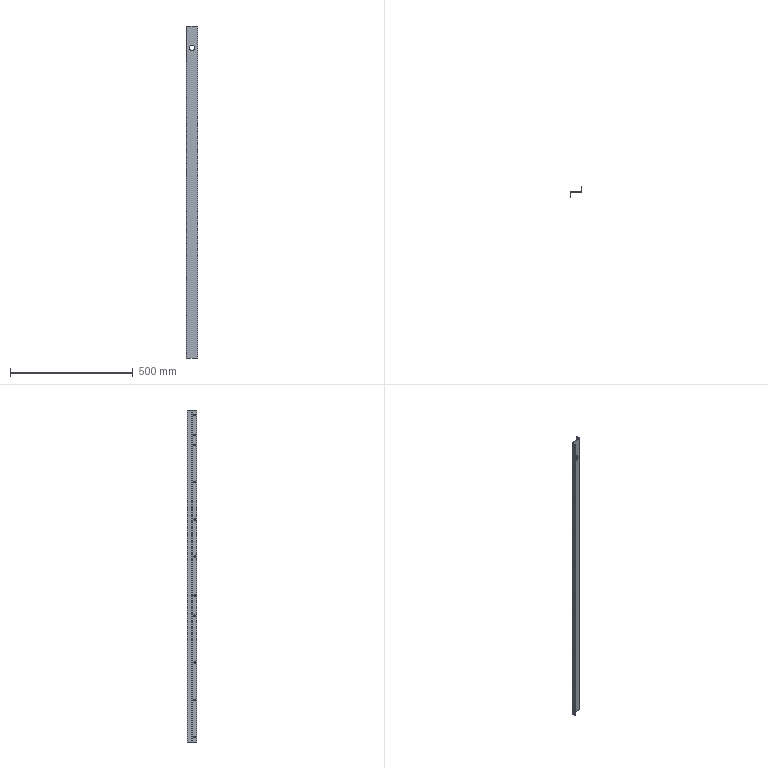Part | SolidWorks | features Cut 3, FlatPattern 1, SMBaseFlange 1, SheetMetal 1 | 1 solid | 46 faces | box 47.2 x 40 x 1350 mm | volume 135924 mm3 | cylinder 28 | plane 18 | commonest cylinder face diameters 6.5 x20 2.4 x2 4.8 x2 6.393 x2 22 x2
STEP:
#1=CARTESIAN_POINT('',(23.9,20.,1250.));
#2=VERTEX_POINT('',#1);
#3=CARTESIAN_POINT('',(23.9,20.,1272.));
#4=VERTEX_POINT('',#3);
#5=CARTESIAN_POINT('',(23.9,20.,1261.));
#6=DIRECTION('',(0.,1.,0.));
#7=DIRECTION('',(0.,0.,1.));
#8=AXIS2_PLACEMENT_3D('',#5,#6,#7);
#9=CIRCLE('',#8,11.);
#10=EDGE_CURVE('',#2,#4,#9,.T.);
#11=ORIENTED_EDGE('',*,*,#10,.T.);
#12=CARTESIAN_POINT('',(23.9,18.8,1272.));
#13=VERTEX_POINT('',#12);
#14=CARTESIAN_POINT('',(23.9,20.8,1272.));
#15=DIRECTION('',(0.,-1.,0.));
#16=VECTOR('',#15,1000.);
#17=LINE('',#14,#16);
#18=EDGE_CURVE('',#4,#13,#17,.T.);
#19=ORIENTED_EDGE('',*,*,#18,.T.);
#20=CARTESIAN_POINT('',(23.9,18.8,1250.));
#21=VERTEX_POINT('',#20);
#22=CARTESIAN_POINT('',(23.9,18.8,1261.));
#23=DIRECTION('',(0.,-1.,0.));
#24=DIRECTION('',(0.,0.,-1.));
#25=AXIS2_PLACEMENT_3D('',#22,#23,#24);
#26=CIRCLE('',#25,11.);
#27=EDGE_CURVE('',#13,#21,#26,.T.);
#28=ORIENTED_EDGE('',*,*,#27,.T.);
#29=CARTESIAN_POINT('',(23.9,20.8,1250.));
#30=DIRECTION('',(0.,-1.,0.));
#31=VECTOR('',#30,1000.);
#32=LINE('',#29,#31);
#33=EDGE_CURVE('',#2,#21,#32,.T.);
#34=ORIENTED_EDGE('',*,*,#33,.F.);
#35=EDGE_LOOP('',(#11,#19,#28,#34));
#36=FACE_OUTER_BOUND('',#35,.T.);
#37=CARTESIAN_POINT('',(23.9,20.8,1261.));
#38=DIRECTION('',(0.,-1.,0.));
#39=DIRECTION('',(0.,0.,-1.));
#40=AXIS2_PLACEMENT_3D('',#37,#38,#39);
#41=CYLINDRICAL_SURFACE('',#40,11.);
#42=ADVANCED_FACE('',(#36),#41,.F.);
#43=CARTESIAN_POINT('',(0.,9.,16.75));
#44=VERTEX_POINT('',#43);
#45=CARTESIAN_POINT('',(0.,9.,23.25));
#46=VERTEX_POINT('',#45);
#47=CARTESIAN_POINT('',(0.,9.,20.));
#48=DIRECTION('',(-1.,0.,0.));
#49=DIRECTION('',(0.,0.,1.));
#50=AXIS2_PLACEMENT_3D('',#47,#48,#49);
#51=CIRCLE('',#50,3.25);
#52=EDGE_CURVE('',#44,#46,#51,.T.);
#53=ORIENTED_EDGE('',*,*,#52,.T.);
#54=CARTESIAN_POINT('',(1.2,9.,23.25));
#55=VERTEX_POINT('',#54);
#56=CARTESIAN_POINT('',(-8.8,9.,23.25));
#57=DIRECTION('',(1.,0.,0.));
#58=VECTOR('',#57,1000.);
#59=LINE('',#56,#58);
#60=EDGE_CURVE('',#46,#55,#59,.T.);
#61=ORIENTED_EDGE('',*,*,#60,.T.);
#62=CARTESIAN_POINT('',(1.2,9.,16.75));
#63=VERTEX_POINT('',#62);
#64=CARTESIAN_POINT('',(1.2,9.,20.));
#65=DIRECTION('',(1.,0.,0.));
#66=DIRECTION('',(0.,0.,1.));
#67=AXIS2_PLACEMENT_3D('',#64,#65,#66);
#68=CIRCLE('',#67,3.25);
#69=EDGE_CURVE('',#55,#63,#68,.T.);
#70=ORIENTED_EDGE('',*,*,#69,.T.);
#71=CARTESIAN_POINT('',(-8.8,9.,16.75));
#72=DIRECTION('',(1.,0.,0.));
#73=VECTOR('',#72,1000.);
#74=LINE('',#71,#73);
#75=EDGE_CURVE('',#44,#63,#74,.T.);
#76=ORIENTED_EDGE('',*,*,#75,.F.);
#77=EDGE_LOOP('',(#53,#61,#70,#76));
#78=FACE_OUTER_BOUND('',#77,.T.);
#79=CARTESIAN_POINT('',(-8.8,9.,20.));
#80=DIRECTION('',(1.,0.,0.));
#81=DIRECTION('',(0.,0.,-1.));
#82=AXIS2_PLACEMENT_3D('',#79,#80,#81);
#83=CYLINDRICAL_SURFACE('',#82,3.25);
#84=ADVANCED_FACE('',(#78),#83,.F.);
#85=CARTESIAN_POINT('',(0.,9.,166.75));
#86=VERTEX_POINT('',#85);
#87=CARTESIAN_POINT('',(0.,9.,173.25));
#88=VERTEX_POINT('',#87);
#89=CARTESIAN_POINT('',(0.,9.,170.));
#90=DIRECTION('',(-1.,0.,0.));
#91=DIRECTION('',(0.,0.,1.));
#92=AXIS2_PLACEMENT_3D('',#89,#90,#91);
#93=CIRCLE('',#92,3.25);
#94=EDGE_CURVE('',#86,#88,#93,.T.);
#95=ORIENTED_EDGE('',*,*,#94,.T.);
#96=CARTESIAN_POINT('',(1.2,9.,173.25));
#97=VERTEX_POINT('',#96);
#98=CARTESIAN_POINT('',(-8.8,9.,173.25));
#99=DIRECTION('',(1.,0.,0.));
#100=VECTOR('',#99,1000.);
#101=LINE('',#98,#100);
#102=EDGE_CURVE('',#88,#97,#101,.T.);
#103=ORIENTED_EDGE('',*,*,#102,.T.);
#104=CARTESIAN_POINT('',(1.2,9.,166.75));
#105=VERTEX_POINT('',#104);
#106=CARTESIAN_POINT('',(1.2,9.,170.));
#107=DIRECTION('',(1.,0.,0.));
#108=DIRECTION('',(0.,0.,1.));
#109=AXIS2_PLACEMENT_3D('',#106,#107,#108);
#110=CIRCLE('',#109,3.25);
#111=EDGE_CURVE('',#97,#105,#110,.T.);
#112=ORIENTED_EDGE('',*,*,#111,.T.);
#113=CARTESIAN_POINT('',(-8.8,9.,166.75));
#114=DIRECTION('',(1.,0.,0.));
#115=VECTOR('',#114,1000.);
#116=LINE('',#113,#115);
#117=EDGE_CURVE('',#86,#105,#116,.T.);
#118=ORIENTED_EDGE('',*,*,#117,.F.);
#119=EDGE_LOOP('',(#95,#103,#112,#118));
#120=FACE_OUTER_BOUND('',#119,.T.);
#121=CARTESIAN_POINT('',(-8.8,9.,170.));
#122=DIRECTION('',(1.,0.,0.));
#123=DIRECTION('',(0.,0.,-1.));
#124=AXIS2_PLACEMENT_3D('',#121,#122,#123);
#125=CYLINDRICAL_SURFACE('',#124,3.25);
#126=ADVANCED_FACE('',(#120),#125,.F.);
#127=CARTESIAN_POINT('',(0.,9.,319.75));
#128=VERTEX_POINT('',#127);
#129=CARTESIAN_POINT('',(0.,9.,326.25));
#130=VERTEX_POINT('',#129);
#131=CARTESIAN_POINT('',(0.,9.,323.));
#132=DIRECTION('',(-1.,0.,0.));
#133=DIRECTION('',(0.,0.,1.));
#134=AXIS2_PLACEMENT_3D('',#131,#132,#133);
#135=CIRCLE('',#134,3.25);
#136=EDGE_CURVE('',#128,#130,#135,.T.);
#137=ORIENTED_EDGE('',*,*,#136,.T.);
#138=CARTESIAN_POINT('',(1.2,9.,326.25));
#139=VERTEX_POINT('',#138);
#140=CARTESIAN_POINT('',(-8.8,9.,326.25));
#141=DIRECTION('',(1.,0.,0.));
#142=VECTOR('',#141,1000.);
#143=LINE('',#140,#142);
#144=EDGE_CURVE('',#130,#139,#143,.T.);
#145=ORIENTED_EDGE('',*,*,#144,.T.);
#146=CARTESIAN_POINT('',(1.2,9.,319.75));
#147=VERTEX_POINT('',#146);
#148=CARTESIAN_POINT('',(1.2,9.,323.));
#149=DIRECTION('',(1.,0.,0.));
#150=DIRECTION('',(0.,0.,1.));
#151=AXIS2_PLACEMENT_3D('',#148,#149,#150);
#152=CIRCLE('',#151,3.25);
#153=EDGE_CURVE('',#139,#147,#152,.T.);
#154=ORIENTED_EDGE('',*,*,#153,.T.);
#155=CARTESIAN_POINT('',(-8.8,9.,319.75));
#156=DIRECTION('',(1.,0.,0.));
#157=VECTOR('',#156,1000.);
#158=LINE('',#155,#157);
#159=EDGE_CURVE('',#128,#147,#158,.T.);
#160=ORIENTED_EDGE('',*,*,#159,.F.);
#161=EDGE_LOOP('',(#137,#145,#154,#160));
#162=FACE_OUTER_BOUND('',#161,.T.);
#163=CARTESIAN_POINT('',(-8.8,9.,323.));
#164=DIRECTION('',(1.,0.,0.));
#165=DIRECTION('',(0.,0.,-1.));
#166=AXIS2_PLACEMENT_3D('',#163,#164,#165);
#167=CYLINDRICAL_SURFACE('',#166,3.25);
#168=ADVANCED_FACE('',(#162),#167,.F.);
#169=CARTESIAN_POINT('',(0.,9.,510.25));
#170=VERTEX_POINT('',#169);
#171=CARTESIAN_POINT('',(0.,9.,516.75));
#172=VERTEX_POINT('',#171);
#173=CARTESIAN_POINT('',(0.,9.,513.5));
#174=DIRECTION('',(-1.,0.,0.));
#175=DIRECTION('',(0.,0.,1.));
#176=AXIS2_PLACEMENT_3D('',#173,#174,#175);
#177=CIRCLE('',#176,3.25);
#178=EDGE_CURVE('',#170,#172,#177,.T.);
#179=ORIENTED_EDGE('',*,*,#178,.T.);
#180=CARTESIAN_POINT('',(1.2,9.,516.75));
#181=VERTEX_POINT('',#180);
#182=CARTESIAN_POINT('',(-8.8,9.,516.75));
#183=DIRECTION('',(1.,0.,0.));
#184=VECTOR('',#183,1000.);
#185=LINE('',#182,#184);
#186=EDGE_CURVE('',#172,#181,#185,.T.);
#187=ORIENTED_EDGE('',*,*,#186,.T.);
#188=CARTESIAN_POINT('',(1.2,9.,510.25));
#189=VERTEX_POINT('',#188);
#190=CARTESIAN_POINT('',(1.2,9.,513.5));
#191=DIRECTION('',(1.,0.,0.));
#192=DIRECTION('',(0.,0.,1.));
#193=AXIS2_PLACEMENT_3D('',#190,#191,#192);
#194=CIRCLE('',#193,3.25);
#195=EDGE_CURVE('',#181,#189,#194,.T.);
#196=ORIENTED_EDGE('',*,*,#195,.T.);
#197=CARTESIAN_POINT('',(-8.8,9.,510.25));
#198=DIRECTION('',(1.,0.,0.));
#199=VECTOR('',#198,1000.);
#200=LINE('',#197,#199);
#201=EDGE_CURVE('',#170,#189,#200,.T.);
#202=ORIENTED_EDGE('',*,*,#201,.F.);
#203=EDGE_LOOP('',(#179,#187,#196,#202));
#204=FACE_OUTER_BOUND('',#203,.T.);
#205=CARTESIAN_POINT('',(-8.8,9.,513.5));
#206=DIRECTION('',(1.,0.,0.));
#207=DIRECTION('',(0.,0.,-1.));
#208=AXIS2_PLACEMENT_3D('',#205,#206,#207);
#209=CYLINDRICAL_SURFACE('',#208,3.25);
#210=ADVANCED_FACE('',(#204),#209,.F.);
#211=CARTESIAN_POINT('',(0.,9.,901.75));
#212=VERTEX_POINT('',#211);
#213=CARTESIAN_POINT('',(0.,9.,908.25));
#214=VERTEX_POINT('',#213);
#215=CARTESIAN_POINT('',(0.,9.,905.));
#216=DIRECTION('',(-1.,0.,0.));
#217=DIRECTION('',(0.,0.,1.));
#218=AXIS2_PLACEMENT_3D('',#215,#216,#217);
#219=CIRCLE('',#218,3.25);
#220=EDGE_CURVE('',#212,#214,#219,.T.);
#221=ORIENTED_EDGE('',*,*,#220,.T.);
#222=CARTESIAN_POINT('',(1.2,9.,908.25));
#223=VERTEX_POINT('',#222);
#224=CARTESIAN_POINT('',(-8.8,9.,908.25));
#225=DIRECTION('',(1.,0.,0.));
#226=VECTOR('',#225,1000.);
#227=LINE('',#224,#226);
#228=EDGE_CURVE('',#214,#223,#227,.T.);
#229=ORIENTED_EDGE('',*,*,#228,.T.);
#230=CARTESIAN_POINT('',(1.2,9.,901.75));
#231=VERTEX_POINT('',#230);
#232=CARTESIAN_POINT('',(1.2,9.,905.));
#233=DIRECTION('',(1.,0.,0.));
#234=DIRECTION('',(0.,0.,1.));
#235=AXIS2_PLACEMENT_3D('',#232,#233,#234);
#236=CIRCLE('',#235,3.25);
#237=EDGE_CURVE('',#223,#231,#236,.T.);
#238=ORIENTED_EDGE('',*,*,#237,.T.);
#239=CARTESIAN_POINT('',(-8.8,9.,901.75));
#240=DIRECTION('',(1.,0.,0.));
#241=VECTOR('',#240,1000.);
#242=LINE('',#239,#241);
#243=EDGE_CURVE('',#212,#231,#242,.T.);
#244=ORIENTED_EDGE('',*,*,#243,.F.);
#245=EDGE_LOOP('',(#221,#229,#238,#244));
#246=FACE_OUTER_BOUND('',#245,.T.);
#247=CARTESIAN_POINT('',(-8.8,9.,905.));
#248=DIRECTION('',(1.,0.,0.));
#249=DIRECTION('',(0.,0.,-1.));
#250=AXIS2_PLACEMENT_3D('',#247,#248,#249);
#251=CYLINDRICAL_SURFACE('',#250,3.25);
#252=ADVANCED_FACE('',(#246),#251,.F.);
#253=CARTESIAN_POINT('',(0.,9.,1054.75));
#254=VERTEX_POINT('',#253);
#255=CARTESIAN_POINT('',(0.,9.,1061.25));
#256=VERTEX_POINT('',#255);
#257=CARTESIAN_POINT('',(0.,9.,1058.));
#258=DIRECTION('',(-1.,0.,0.));
#259=DIRECTION('',(0.,0.,1.));
#260=AXIS2_PLACEMENT_3D('',#257,#258,#259);
#261=CIRCLE('',#260,3.25);
#262=EDGE_CURVE('',#254,#256,#261,.T.);
#263=ORIENTED_EDGE('',*,*,#262,.T.);
#264=CARTESIAN_POINT('',(1.2,9.,1061.25));
#265=VERTEX_POINT('',#264);
#266=CARTESIAN_POINT('',(-8.8,9.,1061.25));
#267=DIRECTION('',(1.,0.,0.));
#268=VECTOR('',#267,1000.);
#269=LINE('',#266,#268);
#270=EDGE_CURVE('',#256,#265,#269,.T.);
#271=ORIENTED_EDGE('',*,*,#270,.T.);
#272=CARTESIAN_POINT('',(1.2,9.,1054.75));
#273=VERTEX_POINT('',#272);
#274=CARTESIAN_POINT('',(1.2,9.,1058.));
#275=DIRECTION('',(1.,0.,0.));
#276=DIRECTION('',(0.,0.,1.));
#277=AXIS2_PLACEMENT_3D('',#274,#275,#276);
#278=CIRCLE('',#277,3.25);
#279=EDGE_CURVE('',#265,#273,#278,.T.);
#280=ORIENTED_EDGE('',*,*,#279,.T.);
#281=CARTESIAN_POINT('',(-8.8,9.,1054.75));
#282=DIRECTION('',(1.,0.,0.));
#283=VECTOR('',#282,1000.);
#284=LINE('',#281,#283);
#285=EDGE_CURVE('',#254,#273,#284,.T.);
#286=ORIENTED_EDGE('',*,*,#285,.F.);
#287=EDGE_LOOP('',(#263,#271,#280,#286));
#288=FACE_OUTER_BOUND('',#287,.T.);
#289=CARTESIAN_POINT('',(-8.8,9.,1058.));
#290=DIRECTION('',(1.,0.,0.));
#291=DIRECTION('',(0.,0.,-1.));
#292=AXIS2_PLACEMENT_3D('',#289,#290,#291);
#293=CYLINDRICAL_SURFACE('',#292,3.25);
#294=ADVANCED_FACE('',(#288),#293,.F.);
#295=CARTESIAN_POINT('',(0.,9.,1204.75));
#296=VERTEX_POINT('',#295);
#297=CARTESIAN_POINT('',(0.,9.,1211.25));
#298=VERTEX_POINT('',#297);
#299=CARTESIAN_POINT('',(0.,9.,1208.));
#300=DIRECTION('',(-1.,0.,0.));
#301=DIRECTION('',(0.,0.,1.));
#302=AXIS2_PLACEMENT_3D('',#299,#300,#301);
#303=CIRCLE('',#302,3.25);
#304=EDGE_CURVE('',#296,#298,#303,.T.);
#305=ORIENTED_EDGE('',*,*,#304,.T.);
#306=CARTESIAN_POINT('',(1.2,9.,1211.25));
#307=VERTEX_POINT('',#306);
#308=CARTESIAN_POINT('',(-8.8,9.,1211.25));
#309=DIRECTION('',(1.,0.,0.));
#310=VECTOR('',#309,1000.);
#311=LINE('',#308,#310);
#312=EDGE_CURVE('',#298,#307,#311,.T.);
#313=ORIENTED_EDGE('',*,*,#312,.T.);
#314=CARTESIAN_POINT('',(1.2,9.,1204.75));
#315=VERTEX_POINT('',#314);
#316=CARTESIAN_POINT('',(1.2,9.,1208.));
#317=DIRECTION('',(1.,0.,0.));
#318=DIRECTION('',(0.,0.,1.));
#319=AXIS2_PLACEMENT_3D('',#316,#317,#318);
#320=CIRCLE('',#319,3.25);
#321=EDGE_CURVE('',#307,#315,#320,.T.);
#322=ORIENTED_EDGE('',*,*,#321,.T.);
#323=CARTESIAN_POINT('',(-8.8,9.,1204.75));
#324=DIRECTION('',(1.,0.,0.));
#325=VECTOR('',#324,1000.);
#326=LINE('',#323,#325);
#327=EDGE_CURVE('',#296,#315,#326,.T.);
#328=ORIENTED_EDGE('',*,*,#327,.F.);
#329=EDGE_LOOP('',(#305,#313,#322,#328));
#330=FACE_OUTER_BOUND('',#329,.T.);
#331=CARTESIAN_POINT('',(-8.8,9.,1208.));
#332=DIRECTION('',(1.,0.,0.));
#333=DIRECTION('',(0.,0.,-1.));
#334=AXIS2_PLACEMENT_3D('',#331,#332,#333);
#335=CYLINDRICAL_SURFACE('',#334,3.25);
#336=ADVANCED_FACE('',(#330),#335,.F.);
#337=CARTESIAN_POINT('',(0.,9.,592.25));
#338=VERTEX_POINT('',#337);
#339=CARTESIAN_POINT('',(0.,9.,598.75));
#340=VERTEX_POINT('',#339);
#341=CARTESIAN_POINT('',(0.,9.,595.5));
#342=DIRECTION('',(-1.,0.,0.));
#343=DIRECTION('',(0.,0.,1.));
#344=AXIS2_PLACEMENT_3D('',#341,#342,#343);
#345=CIRCLE('',#344,3.25);
#346=EDGE_CURVE('',#338,#340,#345,.T.);
#347=ORIENTED_EDGE('',*,*,#346,.T.);
#348=CARTESIAN_POINT('',(1.2,9.,598.75));
#349=VERTEX_POINT('',#348);
#350=CARTESIAN_POINT('',(-8.8,9.,598.75));
#351=DIRECTION('',(1.,0.,0.));
#352=VECTOR('',#351,1000.);
#353=LINE('',#350,#352);
#354=EDGE_CURVE('',#340,#349,#353,.T.);
#355=ORIENTED_EDGE('',*,*,#354,.T.);
#356=CARTESIAN_POINT('',(1.2,9.,592.25));
#357=VERTEX_POINT('',#356);
#358=CARTESIAN_POINT('',(1.2,9.,595.5));
#359=DIRECTION('',(1.,0.,0.));
#360=DIRECTION('',(0.,0.,1.));
#361=AXIS2_PLACEMENT_3D('',#358,#359,#360);
#362=CIRCLE('',#361,3.25);
#363=EDGE_CURVE('',#349,#357,#362,.T.);
#364=ORIENTED_EDGE('',*,*,#363,.T.);
#365=CARTESIAN_POINT('',(-8.8,9.,592.25));
#366=DIRECTION('',(1.,0.,0.));
#367=VECTOR('',#366,1000.);
#368=LINE('',#365,#367);
#369=EDGE_CURVE('',#338,#357,#368,.T.);
#370=ORIENTED_EDGE('',*,*,#369,.F.);
#371=EDGE_LOOP('',(#347,#355,#364,#370));
#372=FACE_OUTER_BOUND('',#371,.T.);
#373=CARTESIAN_POINT('',(-8.8,9.,595.5));
#374=DIRECTION('',(1.,0.,0.));
#375=DIRECTION('',(0.,0.,-1.));
#376=AXIS2_PLACEMENT_3D('',#373,#374,#375);
#377=CYLINDRICAL_SURFACE('',#376,3.25);
#378=ADVANCED_FACE('',(#372),#377,.F.);
#379=CARTESIAN_POINT('',(0.,9.,751.803));
#380=VERTEX_POINT('',#379);
#381=CARTESIAN_POINT('',(0.,9.,758.197));
#382=VERTEX_POINT('',#381);
#383=CARTESIAN_POINT('',(0.,9.,755.));
#384=DIRECTION('',(-1.,0.,0.));
#385=DIRECTION('',(0.,0.,1.));
#386=AXIS2_PLACEMENT_3D('',#383,#384,#385);
#387=CIRCLE('',#386,3.197);
#388=EDGE_CURVE('',#380,#382,#387,.T.);
#389=ORIENTED_EDGE('',*,*,#388,.T.);
#390=CARTESIAN_POINT('',(1.2,9.,758.197));
#391=VERTEX_POINT('',#390);
#392=CARTESIAN_POINT('',(-8.8,9.,758.197));
#393=DIRECTION('',(1.,0.,0.));
#394=VECTOR('',#393,1000.);
#395=LINE('',#392,#394);
#396=EDGE_CURVE('',#382,#391,#395,.T.);
#397=ORIENTED_EDGE('',*,*,#396,.T.);
#398=CARTESIAN_POINT('',(1.2,9.,751.803));
#399=VERTEX_POINT('',#398);
#400=CARTESIAN_POINT('',(1.2,9.,755.));
#401=DIRECTION('',(1.,0.,0.));
#402=DIRECTION('',(0.,0.,1.));
#403=AXIS2_PLACEMENT_3D('',#400,#401,#402);
#404=CIRCLE('',#403,3.197);
#405=EDGE_CURVE('',#391,#399,#404,.T.);
#406=ORIENTED_EDGE('',*,*,#405,.T.);
#407=CARTESIAN_POINT('',(-8.8,9.,751.803));
#408=DIRECTION('',(1.,0.,0.));
#409=VECTOR('',#408,1000.);
#410=LINE('',#407,#409);
#411=EDGE_CURVE('',#380,#399,#410,.T.);
#412=ORIENTED_EDGE('',*,*,#411,.F.);
#413=EDGE_LOOP('',(#389,#397,#406,#412));
#414=FACE_OUTER_BOUND('',#413,.T.);
#415=CARTESIAN_POINT('',(-8.8,9.,755.));
#416=DIRECTION('',(1.,0.,0.));
#417=DIRECTION('',(0.,0.,-1.));
#418=AXIS2_PLACEMENT_3D('',#415,#416,#417);
#419=CYLINDRICAL_SURFACE('',#418,3.197);
#420=ADVANCED_FACE('',(#414),#419,.F.);
#421=CARTESIAN_POINT('',(1.2,12.25,1248.5));
#422=VERTEX_POINT('',#421);
#423=CARTESIAN_POINT('',(1.2,5.75,1248.5));
#424=VERTEX_POINT('',#423);
#425=CARTESIAN_POINT('',(1.2,9.,1248.5));
#426=DIRECTION('',(-1.,0.,0.));
#427=DIRECTION('',(0.,0.,1.));
#428=AXIS2_PLACEMENT_3D('',#425,#426,#427);
#429=CIRCLE('',#428,3.25);
#430=EDGE_CURVE('',#422,#424,#429,.T.);
#431=ORIENTED_EDGE('',*,*,#430,.F.);
#432=CARTESIAN_POINT('',(0.,12.25,1248.5));
#433=VERTEX_POINT('',#432);
#434=CARTESIAN_POINT('',(9.2,12.25,1248.5));
#435=DIRECTION('',(-1.,0.,0.));
#436=VECTOR('',#435,1000.);
#437=LINE('',#434,#436);
#438=EDGE_CURVE('',#422,#433,#437,.T.);
#439=ORIENTED_EDGE('',*,*,#438,.T.);
#440=CARTESIAN_POINT('',(0.,5.75,1248.5));
#441=VERTEX_POINT('',#440);
#442=CARTESIAN_POINT('',(0.,9.,1248.5));
#443=DIRECTION('',(-1.,0.,0.));
#444=DIRECTION('',(0.,0.,1.));
#445=AXIS2_PLACEMENT_3D('',#442,#443,#444);
#446=CIRCLE('',#445,3.25);
#447=EDGE_CURVE('',#433,#441,#446,.T.);
#448=ORIENTED_EDGE('',*,*,#447,.T.);
#449=CARTESIAN_POINT('',(9.2,5.75,1248.5));
#450=DIRECTION('',(-1.,0.,0.));
#451=VECTOR('',#450,1000.);
#452=LINE('',#449,#451);
#453=EDGE_CURVE('',#424,#441,#452,.T.);
#454=ORIENTED_EDGE('',*,*,#453,.F.);
#455=EDGE_LOOP('',(#431,#439,#448,#454));
#456=FACE_OUTER_BOUND('',#455,.T.);
#457=CARTESIAN_POINT('',(9.2,9.,1248.5));
#458=DIRECTION('',(-1.,0.,0.));
#459=DIRECTION('',(0.,-1.,0.));
#460=AXIS2_PLACEMENT_3D('',#457,#458,#459);
#461=CYLINDRICAL_SURFACE('',#460,3.25);
#462=ADVANCED_FACE('',(#456),#461,.F.);
#463=CARTESIAN_POINT('',(1.2,12.25,1330.5));
#464=VERTEX_POINT('',#463);
#465=CARTESIAN_POINT('',(1.2,5.75,1330.5));
#466=VERTEX_POINT('',#465);
#467=CARTESIAN_POINT('',(1.2,9.,1330.5));
#468=DIRECTION('',(-1.,0.,0.));
#469=DIRECTION('',(0.,0.,1.));
#470=AXIS2_PLACEMENT_3D('',#467,#468,#469);
#471=CIRCLE('',#470,3.25);
#472=EDGE_CURVE('',#464,#466,#471,.T.);
#473=ORIENTED_EDGE('',*,*,#472,.F.);
#474=CARTESIAN_POINT('',(0.,12.25,1330.5));
#475=VERTEX_POINT('',#474);
#476=CARTESIAN_POINT('',(9.2,12.25,1330.5));
#477=DIRECTION('',(-1.,0.,0.));
#478=VECTOR('',#477,1000.);
#479=LINE('',#476,#478);
#480=EDGE_CURVE('',#464,#475,#479,.T.);
#481=ORIENTED_EDGE('',*,*,#480,.T.);
#482=CARTESIAN_POINT('',(0.,5.75,1330.5));
#483=VERTEX_POINT('',#482);
#484=CARTESIAN_POINT('',(0.,9.,1330.5));
#485=DIRECTION('',(-1.,0.,0.));
#486=DIRECTION('',(0.,0.,1.));
#487=AXIS2_PLACEMENT_3D('',#484,#485,#486);
#488=CIRCLE('',#487,3.25);
#489=EDGE_CURVE('',#475,#483,#488,.T.);
#490=ORIENTED_EDGE('',*,*,#489,.T.);
#491=CARTESIAN_POINT('',(9.2,5.75,1330.5));
#492=DIRECTION('',(-1.,0.,0.));
#493=VECTOR('',#492,1000.);
#494=LINE('',#491,#493);
#495=EDGE_CURVE('',#466,#483,#494,.T.);
#496=ORIENTED_EDGE('',*,*,#495,.F.);
#497=EDGE_LOOP('',(#473,#481,#490,#496));
#498=FACE_OUTER_BOUND('',#497,.T.);
#499=CARTESIAN_POINT('',(9.2,9.,1330.5));
#500=DIRECTION('',(-1.,0.,0.));
#501=DIRECTION('',(0.,-1.,0.));
#502=AXIS2_PLACEMENT_3D('',#499,#500,#501);
#503=CYLINDRICAL_SURFACE('',#502,3.25);
#504=ADVANCED_FACE('',(#498),#503,.F.);
#505=CARTESIAN_POINT('',(2.4,20.,1350.));
#506=VERTEX_POINT('',#505);
#507=CARTESIAN_POINT('',(2.4,18.8,1350.));
#508=VERTEX_POINT('',#507);
#509=CARTESIAN_POINT('',(2.4,20.,1350.));
#510=DIRECTION('',(0.,-1.,0.));
#511=VECTOR('',#510,1000.);
#512=LINE('',#509,#511);
#513=EDGE_CURVE('',#506,#508,#512,.T.);
#514=ORIENTED_EDGE('',*,*,#513,.F.);
#515=CARTESIAN_POINT('',(0.,17.6,1350.));
#516=VERTEX_POINT('',#515);
#517=CARTESIAN_POINT('',(2.4,17.6,1350.));
#518=DIRECTION('',(0.,0.,-1.));
#519=DIRECTION('',(1.,0.,0.));
#520=AXIS2_PLACEMENT_3D('',#517,#518,#519);
#521=CIRCLE('',#520,2.4);
#522=EDGE_CURVE('',#516,#506,#521,.T.);
#523=ORIENTED_EDGE('',*,*,#522,.F.);
#524=CARTESIAN_POINT('',(1.2,17.6,1350.));
#525=VERTEX_POINT('',#524);
#526=CARTESIAN_POINT('',(1.2,17.6,1350.));
#527=DIRECTION('',(-1.,0.,0.));
#528=VECTOR('',#527,1000.);
#529=LINE('',#526,#528);
#530=EDGE_CURVE('',#525,#516,#529,.T.);
#531=ORIENTED_EDGE('',*,*,#530,.F.);
#532=CARTESIAN_POINT('',(2.4,17.6,1350.));
#533=DIRECTION('',(0.,0.,-1.));
#534=DIRECTION('',(1.,0.,0.));
#535=AXIS2_PLACEMENT_3D('',#532,#533,#534);
#536=CIRCLE('',#535,1.2);
#537=EDGE_CURVE('',#525,#508,#536,.T.);
#538=ORIENTED_EDGE('',*,*,#537,.T.);
#539=EDGE_LOOP('',(#514,#523,#531,#538));
#540=FACE_OUTER_BOUND('',#539,.T.);
#541=CARTESIAN_POINT('',(2.4,20.,1350.));
#542=DIRECTION('',(0.,0.,1.));
#543=DIRECTION('',(1.,0.,0.));
#544=AXIS2_PLACEMENT_3D('',#541,#542,#543);
#545=PLANE('',#544);
#546=ADVANCED_FACE('',(#540),#545,.T.);
#547=CARTESIAN_POINT('',(44.8,20.,1350.));
#548=VERTEX_POINT('',#547);
#549=CARTESIAN_POINT('',(0.,20.,1350.));
#550=DIRECTION('',(1.,0.,0.));
#551=VECTOR('',#550,1000.);
#552=LINE('',#549,#551);
#553=EDGE_CURVE('',#506,#548,#552,.T.);
#554=ORIENTED_EDGE('',*,*,#553,.F.);
#555=ORIENTED_EDGE('',*,*,#513,.T.);
#556=CARTESIAN_POINT('',(44.8,18.8,1350.));
#557=VERTEX_POINT('',#556);
#558=CARTESIAN_POINT('',(0.,18.8,1350.));
#559=DIRECTION('',(1.,0.,0.));
#560=VECTOR('',#559,1000.);
#561=LINE('',#558,#560);
#562=EDGE_CURVE('',#508,#557,#561,.T.);
#563=ORIENTED_EDGE('',*,*,#562,.T.);
#564=CARTESIAN_POINT('',(44.8,18.8,1350.));
#565=DIRECTION('',(0.,1.,0.));
#566=VECTOR('',#565,1000.);
#567=LINE('',#564,#566);
#568=EDGE_CURVE('',#557,#548,#567,.T.);
#569=ORIENTED_EDGE('',*,*,#568,.T.);
#570=EDGE_LOOP('',(#554,#555,#563,#569));
#571=FACE_OUTER_BOUND('',#570,.T.);
#572=CARTESIAN_POINT('',(1.2,17.6,1350.));
#573=DIRECTION('',(0.,0.,1.));
#574=DIRECTION('',(1.,0.,0.));
#575=AXIS2_PLACEMENT_3D('',#572,#573,#574);
#576=PLANE('',#575);
#577=ADVANCED_FACE('',(#571),#576,.T.);
#578=CARTESIAN_POINT('',(0.,17.6,0.));
#579=VERTEX_POINT('',#578);
#580=CARTESIAN_POINT('',(1.2,17.6,0.));
#581=VERTEX_POINT('',#580);
#582=CARTESIAN_POINT('',(0.,17.6,0.));
#583=DIRECTION('',(1.,0.,0.));
#584=VECTOR('',#583,1000.);
#585=LINE('',#582,#584);
#586=EDGE_CURVE('',#579,#581,#585,.T.);
#587=ORIENTED_EDGE('',*,*,#586,.F.);
#588=CARTESIAN_POINT('',(2.4,20.,0.));
#589=VERTEX_POINT('',#588);
#590=CARTESIAN_POINT('',(2.4,17.6,0.));
#591=DIRECTION('',(0.,0.,-1.));
#592=DIRECTION('',(1.,0.,0.));
#593=AXIS2_PLACEMENT_3D('',#590,#591,#592);
#594=CIRCLE('',#593,2.4);
#595=EDGE_CURVE('',#579,#589,#594,.T.);
#596=ORIENTED_EDGE('',*,*,#595,.T.);
#597=CARTESIAN_POINT('',(2.4,18.8,0.));
#598=VERTEX_POINT('',#597);
#599=CARTESIAN_POINT('',(2.4,18.8,0.));
#600=DIRECTION('',(0.,1.,0.));
#601=VECTOR('',#600,1000.);
#602=LINE('',#599,#601);
#603=EDGE_CURVE('',#598,#589,#602,.T.);
#604=ORIENTED_EDGE('',*,*,#603,.F.);
#605=CARTESIAN_POINT('',(2.4,17.6,0.));
#606=DIRECTION('',(0.,0.,-1.));
#607=DIRECTION('',(1.,0.,0.));
#608=AXIS2_PLACEMENT_3D('',#605,#606,#607);
#609=CIRCLE('',#608,1.2);
#610=EDGE_CURVE('',#581,#598,#609,.T.);
#611=ORIENTED_EDGE('',*,*,#610,.F.);
#612=EDGE_LOOP('',(#587,#596,#604,#611));
#613=FACE_OUTER_BOUND('',#612,.T.);
#614=CARTESIAN_POINT('',(0.,17.6,0.));
#615=DIRECTION('',(0.,0.,-1.));
#616=DIRECTION('',(-1.,0.,0.));
#617=AXIS2_PLACEMENT_3D('',#614,#615,#616);
#618=PLANE('',#617);
#619=ADVANCED_FACE('',(#613),#618,.T.);
#620=CARTESIAN_POINT('',(0.,0.,0.));
#621=VERTEX_POINT('',#620);
#622=CARTESIAN_POINT('',(0.,0.,0.));
#623=DIRECTION('',(0.,1.,0.));
#624=VECTOR('',#623,1000.);
#625=LINE('',#622,#624);
#626=EDGE_CURVE('',#621,#579,#625,.T.);
#627=ORIENTED_EDGE('',*,*,#626,.T.);
#628=ORIENTED_EDGE('',*,*,#586,.T.);
#629=CARTESIAN_POINT('',(1.2,0.,0.));
#630=VERTEX_POINT('',#629);
#631=CARTESIAN_POINT('',(1.2,0.,0.));
#632=DIRECTION('',(0.,1.,0.));
#633=VECTOR('',#632,1000.);
#634=LINE('',#631,#633);
#635=EDGE_CURVE('',#630,#581,#634,.T.);
#636=ORIENTED_EDGE('',*,*,#635,.F.);
#637=CARTESIAN_POINT('',(1.2,0.,0.));
#638=DIRECTION('',(-1.,0.,0.));
#639=VECTOR('',#638,1000.);
#640=LINE('',#637,#639);
#641=EDGE_CURVE('',#630,#621,#640,.T.);
#642=ORIENTED_EDGE('',*,*,#641,.T.);
#643=EDGE_LOOP('',(#627,#628,#636,#642));
#644=FACE_OUTER_BOUND('',#643,.T.);
#645=CARTESIAN_POINT('',(2.4,18.8,0.));
#646=DIRECTION('',(0.,0.,-1.));
#647=DIRECTION('',(-1.,0.,0.));
#648=AXIS2_PLACEMENT_3D('',#645,#646,#647);
#649=PLANE('',#648);
#650=ADVANCED_FACE('',(#644),#649,.T.);
#651=CARTESIAN_POINT('',(46.,21.2,1350.));
#652=VERTEX_POINT('',#651);
#653=CARTESIAN_POINT('',(47.2,21.2,1350.));
#654=VERTEX_POINT('',#653);
#655=CARTESIAN_POINT('',(46.,21.2,1350.));
#656=DIRECTION('',(1.,0.,0.));
#657=VECTOR('',#656,1000.);
#658=LINE('',#655,#657);
#659=EDGE_CURVE('',#652,#654,#658,.T.);
#660=ORIENTED_EDGE('',*,*,#659,.F.);
#661=CARTESIAN_POINT('',(44.8,21.2,1350.));
#662=DIRECTION('',(0.,0.,1.));
#663=DIRECTION('',(-1.,0.,0.));
#664=AXIS2_PLACEMENT_3D('',#661,#662,#663);
#665=CIRCLE('',#664,1.2);
#666=EDGE_CURVE('',#548,#652,#665,.T.);
#667=ORIENTED_EDGE('',*,*,#666,.F.);
#668=ORIENTED_EDGE('',*,*,#568,.F.);
#669=CARTESIAN_POINT('',(44.8,21.2,1350.));
#670=DIRECTION('',(0.,0.,1.));
#671=DIRECTION('',(1.,0.,0.));
#672=AXIS2_PLACEMENT_3D('',#669,#670,#671);
#673=CIRCLE('',#672,2.4);
#674=EDGE_CURVE('',#557,#654,#673,.T.);
#675=ORIENTED_EDGE('',*,*,#674,.T.);
#676=EDGE_LOOP('',(#660,#667,#668,#675));
#677=FACE_OUTER_BOUND('',#676,.T.);
#678=CARTESIAN_POINT('',(46.,21.2,1350.));
#679=DIRECTION('',(0.,0.,1.));
#680=DIRECTION('',(1.,0.,0.));
#681=AXIS2_PLACEMENT_3D('',#678,#679,#680);
#682=PLANE('',#681);
#683=ADVANCED_FACE('',(#677),#682,.T.);
#684=CARTESIAN_POINT('',(46.,40.,1350.));
#685=VERTEX_POINT('',#684);
#686=CARTESIAN_POINT('',(46.,20.,1350.));
#687=DIRECTION('',(0.,1.,0.));
#688=VECTOR('',#687,1000.);
#689=LINE('',#686,#688);
#690=EDGE_CURVE('',#652,#685,#689,.T.);
#691=ORIENTED_EDGE('',*,*,#690,.F.);
#692=ORIENTED_EDGE('',*,*,#659,.T.);
#693=CARTESIAN_POINT('',(47.2,40.,1350.));
#694=VERTEX_POINT('',#693);
#695=CARTESIAN_POINT('',(47.2,20.,1350.));
#696=DIRECTION('',(0.,1.,0.));
#697=VECTOR('',#696,1000.);
#698=LINE('',#695,#697);
#699=EDGE_CURVE('',#654,#694,#698,.T.);
#700=ORIENTED_EDGE('',*,*,#699,.T.);
#701=CARTESIAN_POINT('',(46.,40.,1350.));
#702=DIRECTION('',(1.,0.,0.));
#703=VECTOR('',#702,1000.);
#704=LINE('',#701,#703);
#705=EDGE_CURVE('',#685,#694,#704,.T.);
#706=ORIENTED_EDGE('',*,*,#705,.F.);
#707=EDGE_LOOP('',(#691,#692,#700,#706));
#708=FACE_OUTER_BOUND('',#707,.T.);
#709=CARTESIAN_POINT('',(44.8,18.8,1350.));
#710=DIRECTION('',(0.,0.,1.));
#711=DIRECTION('',(1.,0.,0.));
#712=AXIS2_PLACEMENT_3D('',#709,#710,#711);
#713=PLANE('',#712);
#714=ADVANCED_FACE('',(#708),#713,.T.);
#715=CARTESIAN_POINT('',(44.8,20.,0.));
#716=VERTEX_POINT('',#715);
#717=CARTESIAN_POINT('',(44.8,18.8,0.));
#718=VERTEX_POINT('',#717);
#719=CARTESIAN_POINT('',(44.8,20.,0.));
#720=DIRECTION('',(0.,-1.,0.));
#721=VECTOR('',#720,1000.);
#722=LINE('',#719,#721);
#723=EDGE_CURVE('',#716,#718,#722,.T.);
#724=ORIENTED_EDGE('',*,*,#723,.F.);
#725=CARTESIAN_POINT('',(46.,21.2,0.));
#726=VERTEX_POINT('',#725);
#727=CARTESIAN_POINT('',(44.8,21.2,0.));
#728=DIRECTION('',(0.,0.,1.));
#729=DIRECTION('',(-1.,0.,0.));
#730=AXIS2_PLACEMENT_3D('',#727,#728,#729);
#731=CIRCLE('',#730,1.2);
#732=EDGE_CURVE('',#716,#726,#731,.T.);
#733=ORIENTED_EDGE('',*,*,#732,.T.);
#734=CARTESIAN_POINT('',(47.2,21.2,0.));
#735=VERTEX_POINT('',#734);
#736=CARTESIAN_POINT('',(47.2,21.2,0.));
#737=DIRECTION('',(-1.,0.,0.));
#738=VECTOR('',#737,1000.);
#739=LINE('',#736,#738);
#740=EDGE_CURVE('',#735,#726,#739,.T.);
#741=ORIENTED_EDGE('',*,*,#740,.F.);
#742=CARTESIAN_POINT('',(44.8,21.2,0.));
#743=DIRECTION('',(0.,0.,1.));
#744=DIRECTION('',(1.,0.,0.));
#745=AXIS2_PLACEMENT_3D('',#742,#743,#744);
#746=CIRCLE('',#745,2.4);
#747=EDGE_CURVE('',#718,#735,#746,.T.);
#748=ORIENTED_EDGE('',*,*,#747,.F.);
#749=EDGE_LOOP('',(#724,#733,#741,#748));
#750=FACE_OUTER_BOUND('',#749,.T.);
#751=CARTESIAN_POINT('',(44.8,20.,0.));
#752=DIRECTION('',(0.,0.,-1.));
#753=DIRECTION('',(-1.,0.,0.));
#754=AXIS2_PLACEMENT_3D('',#751,#752,#753);
#755=PLANE('',#754);
#756=ADVANCED_FACE('',(#750),#755,.T.);
#757=CARTESIAN_POINT('',(0.,20.,0.));
#758=DIRECTION('',(1.,0.,0.));
#759=VECTOR('',#758,1000.);
#760=LINE('',#757,#759);
#761=EDGE_CURVE('',#589,#716,#760,.T.);
#762=ORIENTED_EDGE('',*,*,#761,.T.);
#763=ORIENTED_EDGE('',*,*,#723,.T.);
#764=CARTESIAN_POINT('',(0.,18.8,0.));
#765=DIRECTION('',(1.,0.,0.));
#766=VECTOR('',#765,1000.);
#767=LINE('',#764,#766);
#768=EDGE_CURVE('',#598,#718,#767,.T.);
#769=ORIENTED_EDGE('',*,*,#768,.F.);
#770=ORIENTED_EDGE('',*,*,#603,.T.);
#771=EDGE_LOOP('',(#762,#763,#769,#770));
#772=FACE_OUTER_BOUND('',#771,.T.);
#773=CARTESIAN_POINT('',(47.2,21.2,0.));
#774=DIRECTION('',(0.,0.,-1.));
#775=DIRECTION('',(-1.,0.,0.));
#776=AXIS2_PLACEMENT_3D('',#773,#774,#775);
#777=PLANE('',#776);
#778=ADVANCED_FACE('',(#772),#777,.T.);
#779=CARTESIAN_POINT('',(47.2,40.,0.));
#780=VERTEX_POINT('',#779);
#781=CARTESIAN_POINT('',(47.2,20.,0.));
#782=DIRECTION('',(0.,1.,0.));
#783=VECTOR('',#782,1000.);
#784=LINE('',#781,#783);
#785=EDGE_CURVE('',#735,#780,#784,.T.);
#786=ORIENTED_EDGE('',*,*,#785,.T.);
#787=CARTESIAN_POINT('',(47.2,40.,1350.));
#788=DIRECTION('',(0.,0.,-1.));
#789=VECTOR('',#788,1000.);
#790=LINE('',#787,#789);
#791=EDGE_CURVE('',#694,#780,#790,.T.);
#792=ORIENTED_EDGE('',*,*,#791,.F.);
#793=ORIENTED_EDGE('',*,*,#699,.F.);
#794=CARTESIAN_POINT('',(47.2,21.2,1350.));
#795=DIRECTION('',(0.,0.,-1.));
#796=VECTOR('',#795,1000.);
#797=LINE('',#794,#796);
#798=EDGE_CURVE('',#654,#735,#797,.T.);
#799=ORIENTED_EDGE('',*,*,#798,.T.);
#800=EDGE_LOOP('',(#786,#792,#793,#799));
#801=FACE_OUTER_BOUND('',#800,.T.);
#802=CARTESIAN_POINT('',(47.2,20.,1350.));
#803=DIRECTION('',(-1.,0.,0.));
#804=DIRECTION('',(0.,0.,1.));
#805=AXIS2_PLACEMENT_3D('',#802,#803,#804);
#806=PLANE('',#805);
#807=ADVANCED_FACE('',(#801),#806,.F.);
#808=CARTESIAN_POINT('',(46.,40.,0.));
#809=VERTEX_POINT('',#808);
#810=CARTESIAN_POINT('',(46.,40.,0.));
#811=DIRECTION('',(1.,0.,0.));
#812=VECTOR('',#811,1000.);
#813=LINE('',#810,#812);
#814=EDGE_CURVE('',#809,#780,#813,.T.);
#815=ORIENTED_EDGE('',*,*,#814,.F.);
#816=CARTESIAN_POINT('',(46.,40.,1350.));
#817=DIRECTION('',(0.,0.,-1.));
#818=VECTOR('',#817,1000.);
#819=LINE('',#816,#818);
#820=EDGE_CURVE('',#685,#809,#819,.T.);
#821=ORIENTED_EDGE('',*,*,#820,.F.);
#822=ORIENTED_EDGE('',*,*,#705,.T.);
#823=ORIENTED_EDGE('',*,*,#791,.T.);
#824=EDGE_LOOP('',(#815,#821,#822,#823));
#825=FACE_OUTER_BOUND('',#824,.T.);
#826=CARTESIAN_POINT('',(46.,40.,1350.));
#827=DIRECTION('',(0.,1.,0.));
#828=DIRECTION('',(0.,0.,1.));
#829=AXIS2_PLACEMENT_3D('',#826,#827,#828);
#830=PLANE('',#829);
#831=ADVANCED_FACE('',(#825),#830,.T.);
#832=CARTESIAN_POINT('',(46.,20.,0.));
#833=DIRECTION('',(0.,1.,0.));
#834=VECTOR('',#833,1000.);
#835=LINE('',#832,#834);
#836=EDGE_CURVE('',#726,#809,#835,.T.);
#837=ORIENTED_EDGE('',*,*,#836,.F.);
#838=CARTESIAN_POINT('',(46.,21.2,1350.));
#839=DIRECTION('',(0.,0.,-1.));
#840=VECTOR('',#839,1000.);
#841=LINE('',#838,#840);
#842=EDGE_CURVE('',#652,#726,#841,.T.);
#843=ORIENTED_EDGE('',*,*,#842,.F.);
#844=ORIENTED_EDGE('',*,*,#690,.T.);
#845=ORIENTED_EDGE('',*,*,#820,.T.);
#846=EDGE_LOOP('',(#837,#843,#844,#845));
#847=FACE_OUTER_BOUND('',#846,.T.);
#848=CARTESIAN_POINT('',(46.,20.,1350.));
#849=DIRECTION('',(-1.,0.,0.));
#850=DIRECTION('',(0.,0.,1.));
#851=AXIS2_PLACEMENT_3D('',#848,#849,#850);
#852=PLANE('',#851);
#853=ADVANCED_FACE('',(#847),#852,.T.);
#854=ORIENTED_EDGE('',*,*,#732,.F.);
#855=CARTESIAN_POINT('',(44.8,20.,1350.));
#856=DIRECTION('',(0.,0.,-1.));
#857=VECTOR('',#856,1000.);
#858=LINE('',#855,#857);
#859=EDGE_CURVE('',#548,#716,#858,.T.);
#860=ORIENTED_EDGE('',*,*,#859,.F.);
#861=ORIENTED_EDGE('',*,*,#666,.T.);
#862=ORIENTED_EDGE('',*,*,#842,.T.);
#863=EDGE_LOOP('',(#854,#860,#861,#862));
#864=FACE_OUTER_BOUND('',#863,.T.);
#865=CARTESIAN_POINT('',(44.8,21.2,1350.));
#866=DIRECTION('',(0.,0.,-1.));
#867=DIRECTION('',(-1.,0.,0.));
#868=AXIS2_PLACEMENT_3D('',#865,#866,#867);
#869=CYLINDRICAL_SURFACE('',#868,1.2);
#870=ADVANCED_FACE('',(#864),#869,.F.);
#871=ORIENTED_EDGE('',*,*,#10,.F.);
#872=CARTESIAN_POINT('',(23.9,20.,1261.));
#873=DIRECTION('',(0.,1.,0.));
#874=DIRECTION('',(0.,0.,1.));
#875=AXIS2_PLACEMENT_3D('',#872,#873,#874);
#876=CIRCLE('',#875,11.);
#877=EDGE_CURVE('',#4,#2,#876,.T.);
#878=ORIENTED_EDGE('',*,*,#877,.F.);
#879=EDGE_LOOP('',(#871,#878));
#880=FACE_BOUND('',#879,.T.);
#881=ORIENTED_EDGE('',*,*,#761,.F.);
#882=CARTESIAN_POINT('',(2.4,20.,1350.));
#883=DIRECTION('',(0.,0.,-1.));
#884=VECTOR('',#883,1000.);
#885=LINE('',#882,#884);
#886=EDGE_CURVE('',#506,#589,#885,.T.);
#887=ORIENTED_EDGE('',*,*,#886,.F.);
#888=ORIENTED_EDGE('',*,*,#553,.T.);
#889=ORIENTED_EDGE('',*,*,#859,.T.);
#890=EDGE_LOOP('',(#881,#887,#888,#889));
#891=FACE_OUTER_BOUND('',#890,.T.);
#892=CARTESIAN_POINT('',(0.,20.,1350.));
#893=DIRECTION('',(0.,1.,0.));
#894=DIRECTION('',(0.,0.,1.));
#895=AXIS2_PLACEMENT_3D('',#892,#893,#894);
#896=PLANE('',#895);
#897=ADVANCED_FACE('',(#880,#891),#896,.T.);
#898=ORIENTED_EDGE('',*,*,#595,.F.);
#899=CARTESIAN_POINT('',(0.,17.6,1350.));
#900=DIRECTION('',(0.,0.,-1.));
#901=VECTOR('',#900,1000.);
#902=LINE('',#899,#901);
#903=EDGE_CURVE('',#516,#579,#902,.T.);
#904=ORIENTED_EDGE('',*,*,#903,.F.);
#905=ORIENTED_EDGE('',*,*,#522,.T.);
#906=ORIENTED_EDGE('',*,*,#886,.T.);
#907=EDGE_LOOP('',(#898,#904,#905,#906));
#908=FACE_OUTER_BOUND('',#907,.T.);
#909=CARTESIAN_POINT('',(2.4,17.6,1350.));
#910=DIRECTION('',(0.,0.,-1.));
#911=DIRECTION('',(-1.,0.,0.));
#912=AXIS2_PLACEMENT_3D('',#909,#910,#911);
#913=CYLINDRICAL_SURFACE('',#912,2.4);
#914=ADVANCED_FACE('',(#908),#913,.T.);
#915=ORIENTED_EDGE('',*,*,#52,.F.);
#916=CARTESIAN_POINT('',(0.,9.,20.));
#917=DIRECTION('',(-1.,0.,0.));
#918=DIRECTION('',(0.,0.,1.));
#919=AXIS2_PLACEMENT_3D('',#916,#917,#918);
#920=CIRCLE('',#919,3.25);
#921=EDGE_CURVE('',#46,#44,#920,.T.);
#922=ORIENTED_EDGE('',*,*,#921,.F.);
#923=EDGE_LOOP('',(#915,#922));
#924=FACE_BOUND('',#923,.T.);
#925=ORIENTED_EDGE('',*,*,#94,.F.);
#926=CARTESIAN_POINT('',(0.,9.,170.));
#927=DIRECTION('',(-1.,0.,0.));
#928=DIRECTION('',(0.,0.,1.));
#929=AXIS2_PLACEMENT_3D('',#926,#927,#928);
#930=CIRCLE('',#929,3.25);
#931=EDGE_CURVE('',#88,#86,#930,.T.);
#932=ORIENTED_EDGE('',*,*,#931,.F.);
#933=EDGE_LOOP('',(#925,#932));
#934=FACE_BOUND('',#933,.T.);
#935=ORIENTED_EDGE('',*,*,#136,.F.);
#936=CARTESIAN_POINT('',(0.,9.,323.));
#937=DIRECTION('',(-1.,0.,0.));
#938=DIRECTION('',(0.,0.,1.));
#939=AXIS2_PLACEMENT_3D('',#936,#937,#938);
#940=CIRCLE('',#939,3.25);
#941=EDGE_CURVE('',#130,#128,#940,.T.);
#942=ORIENTED_EDGE('',*,*,#941,.F.);
#943=EDGE_LOOP('',(#935,#942));
#944=FACE_BOUND('',#943,.T.);
#945=ORIENTED_EDGE('',*,*,#178,.F.);
#946=CARTESIAN_POINT('',(0.,9.,513.5));
#947=DIRECTION('',(-1.,0.,0.));
#948=DIRECTION('',(0.,0.,1.));
#949=AXIS2_PLACEMENT_3D('',#946,#947,#948);
#950=CIRCLE('',#949,3.25);
#951=EDGE_CURVE('',#172,#170,#950,.T.);
#952=ORIENTED_EDGE('',*,*,#951,.F.);
#953=EDGE_LOOP('',(#945,#952));
#954=FACE_BOUND('',#953,.T.);
#955=ORIENTED_EDGE('',*,*,#220,.F.);
#956=CARTESIAN_POINT('',(0.,9.,905.));
#957=DIRECTION('',(-1.,0.,0.));
#958=DIRECTION('',(0.,0.,1.));
#959=AXIS2_PLACEMENT_3D('',#956,#957,#958);
#960=CIRCLE('',#959,3.25);
#961=EDGE_CURVE('',#214,#212,#960,.T.);
#962=ORIENTED_EDGE('',*,*,#961,.F.);
#963=EDGE_LOOP('',(#955,#962));
#964=FACE_BOUND('',#963,.T.);
#965=ORIENTED_EDGE('',*,*,#262,.F.);
#966=CARTESIAN_POINT('',(0.,9.,1058.));
#967=DIRECTION('',(-1.,0.,0.));
#968=DIRECTION('',(0.,0.,1.));
#969=AXIS2_PLACEMENT_3D('',#966,#967,#968);
#970=CIRCLE('',#969,3.25);
#971=EDGE_CURVE('',#256,#254,#970,.T.);
#972=ORIENTED_EDGE('',*,*,#971,.F.);
#973=EDGE_LOOP('',(#965,#972));
#974=FACE_BOUND('',#973,.T.);
#975=ORIENTED_EDGE('',*,*,#304,.F.);
#976=CARTESIAN_POINT('',(0.,9.,1208.));
#977=DIRECTION('',(-1.,0.,0.));
#978=DIRECTION('',(0.,0.,1.));
#979=AXIS2_PLACEMENT_3D('',#976,#977,#978);
#980=CIRCLE('',#979,3.25);
#981=EDGE_CURVE('',#298,#296,#980,.T.);
#982=ORIENTED_EDGE('',*,*,#981,.F.);
#983=EDGE_LOOP('',(#975,#982));
#984=FACE_BOUND('',#983,.T.);
#985=ORIENTED_EDGE('',*,*,#346,.F.);
#986=CARTESIAN_POINT('',(0.,9.,595.5));
#987=DIRECTION('',(-1.,0.,0.));
#988=DIRECTION('',(0.,0.,1.));
#989=AXIS2_PLACEMENT_3D('',#986,#987,#988);
#990=CIRCLE('',#989,3.25);
#991=EDGE_CURVE('',#340,#338,#990,.T.);
#992=ORIENTED_EDGE('',*,*,#991,.F.);
#993=EDGE_LOOP('',(#985,#992));
#994=FACE_BOUND('',#993,.T.);
#995=ORIENTED_EDGE('',*,*,#388,.F.);
#996=CARTESIAN_POINT('',(0.,9.,755.));
#997=DIRECTION('',(-1.,0.,0.));
#998=DIRECTION('',(0.,0.,1.));
#999=AXIS2_PLACEMENT_3D('',#996,#997,#998);
#1000=CIRCLE('',#999,3.197);
#1001=EDGE_CURVE('',#382,#380,#1000,.T.);
#1002=ORIENTED_EDGE('',*,*,#1001,.F.);
#1003=EDGE_LOOP('',(#995,#1002));
#1004=FACE_BOUND('',#1003,.T.);
#1005=CARTESIAN_POINT('',(0.,9.,1248.5));
#1006=DIRECTION('',(-1.,0.,0.));
#1007=DIRECTION('',(0.,0.,1.));
#1008=AXIS2_PLACEMENT_3D('',#1005,#1006,#1007);
#1009=CIRCLE('',#1008,3.25);
#1010=EDGE_CURVE('',#441,#433,#1009,.T.);
#1011=ORIENTED_EDGE('',*,*,#1010,.F.);
#1012=ORIENTED_EDGE('',*,*,#447,.F.);
#1013=EDGE_LOOP('',(#1011,#1012));
#1014=FACE_BOUND('',#1013,.T.);
#1015=CARTESIAN_POINT('',(0.,9.,1330.5));
#1016=DIRECTION('',(-1.,0.,0.));
#1017=DIRECTION('',(0.,0.,1.));
#1018=AXIS2_PLACEMENT_3D('',#1015,#1016,#1017);
#1019=CIRCLE('',#1018,3.25);
#1020=EDGE_CURVE('',#483,#475,#1019,.T.);
#1021=ORIENTED_EDGE('',*,*,#1020,.F.);
#1022=ORIENTED_EDGE('',*,*,#489,.F.);
#1023=EDGE_LOOP('',(#1021,#1022));
#1024=FACE_BOUND('',#1023,.T.);
#1025=ORIENTED_EDGE('',*,*,#626,.F.);
#1026=CARTESIAN_POINT('',(0.,0.,1350.));
#1027=VERTEX_POINT('',#1026);
#1028=CARTESIAN_POINT('',(0.,0.,1350.));
#1029=DIRECTION('',(0.,0.,-1.));
#1030=VECTOR('',#1029,1000.);
#1031=LINE('',#1028,#1030);
#1032=EDGE_CURVE('',#1027,#621,#1031,.T.);
#1033=ORIENTED_EDGE('',*,*,#1032,.F.);
#1034=CARTESIAN_POINT('',(0.,0.,1350.));
#1035=DIRECTION('',(0.,1.,0.));
#1036=VECTOR('',#1035,1000.);
#1037=LINE('',#1034,#1036);
#1038=EDGE_CURVE('',#1027,#516,#1037,.T.);
#1039=ORIENTED_EDGE('',*,*,#1038,.T.);
#1040=ORIENTED_EDGE('',*,*,#903,.T.);
#1041=EDGE_LOOP('',(#1025,#1033,#1039,#1040));
#1042=FACE_OUTER_BOUND('',#1041,.T.);
#1043=CARTESIAN_POINT('',(0.,0.,1350.));
#1044=DIRECTION('',(-1.,0.,0.));
#1045=DIRECTION('',(0.,0.,1.));
#1046=AXIS2_PLACEMENT_3D('',#1043,#1044,#1045);
#1047=PLANE('',#1046);
#1048=ADVANCED_FACE('',(#924,#934,#944,#954,#964,#974,#984,#994,#1004,#1014,#1024,#1042),#1047,.T.);
#1049=ORIENTED_EDGE('',*,*,#641,.F.);
#1050=CARTESIAN_POINT('',(1.2,0.,1350.));
#1051=VERTEX_POINT('',#1050);
#1052=CARTESIAN_POINT('',(1.2,0.,1350.));
#1053=DIRECTION('',(0.,0.,-1.));
#1054=VECTOR('',#1053,1000.);
#1055=LINE('',#1052,#1054);
#1056=EDGE_CURVE('',#1051,#630,#1055,.T.);
#1057=ORIENTED_EDGE('',*,*,#1056,.F.);
#1058=CARTESIAN_POINT('',(1.2,0.,1350.));
#1059=DIRECTION('',(-1.,0.,0.));
#1060=VECTOR('',#1059,1000.);
#1061=LINE('',#1058,#1060);
#1062=EDGE_CURVE('',#1051,#1027,#1061,.T.);
#1063=ORIENTED_EDGE('',*,*,#1062,.T.);
#1064=ORIENTED_EDGE('',*,*,#1032,.T.);
#1065=EDGE_LOOP('',(#1049,#1057,#1063,#1064));
#1066=FACE_OUTER_BOUND('',#1065,.T.);
#1067=CARTESIAN_POINT('',(1.2,0.,1350.));
#1068=DIRECTION('',(0.,-1.,0.));
#1069=DIRECTION('',(0.,0.,-1.));
#1070=AXIS2_PLACEMENT_3D('',#1067,#1068,#1069);
#1071=PLANE('',#1070);
#1072=ADVANCED_FACE('',(#1066),#1071,.T.);
#1073=CARTESIAN_POINT('',(1.2,9.,20.));
#1074=DIRECTION('',(1.,0.,0.));
#1075=DIRECTION('',(0.,0.,1.));
#1076=AXIS2_PLACEMENT_3D('',#1073,#1074,#1075);
#1077=CIRCLE('',#1076,3.25);
#1078=EDGE_CURVE('',#63,#55,#1077,.T.);
#1079=ORIENTED_EDGE('',*,*,#1078,.F.);
#1080=ORIENTED_EDGE('',*,*,#69,.F.);
#1081=EDGE_LOOP('',(#1079,#1080));
#1082=FACE_BOUND('',#1081,.T.);
#1083=CARTESIAN_POINT('',(1.2,9.,170.));
#1084=DIRECTION('',(1.,0.,0.));
#1085=DIRECTION('',(0.,0.,1.));
#1086=AXIS2_PLACEMENT_3D('',#1083,#1084,#1085);
#1087=CIRCLE('',#1086,3.25);
#1088=EDGE_CURVE('',#105,#97,#1087,.T.);
#1089=ORIENTED_EDGE('',*,*,#1088,.F.);
#1090=ORIENTED_EDGE('',*,*,#111,.F.);
#1091=EDGE_LOOP('',(#1089,#1090));
#1092=FACE_BOUND('',#1091,.T.);
#1093=CARTESIAN_POINT('',(1.2,9.,323.));
#1094=DIRECTION('',(1.,0.,0.));
#1095=DIRECTION('',(0.,0.,1.));
#1096=AXIS2_PLACEMENT_3D('',#1093,#1094,#1095);
#1097=CIRCLE('',#1096,3.25);
#1098=EDGE_CURVE('',#147,#139,#1097,.T.);
#1099=ORIENTED_EDGE('',*,*,#1098,.F.);
#1100=ORIENTED_EDGE('',*,*,#153,.F.);
#1101=EDGE_LOOP('',(#1099,#1100));
#1102=FACE_BOUND('',#1101,.T.);
#1103=CARTESIAN_POINT('',(1.2,9.,513.5));
#1104=DIRECTION('',(1.,0.,0.));
#1105=DIRECTION('',(0.,0.,1.));
#1106=AXIS2_PLACEMENT_3D('',#1103,#1104,#1105);
#1107=CIRCLE('',#1106,3.25);
#1108=EDGE_CURVE('',#189,#181,#1107,.T.);
#1109=ORIENTED_EDGE('',*,*,#1108,.F.);
#1110=ORIENTED_EDGE('',*,*,#195,.F.);
#1111=EDGE_LOOP('',(#1109,#1110));
#1112=FACE_BOUND('',#1111,.T.);
#1113=CARTESIAN_POINT('',(1.2,9.,905.));
#1114=DIRECTION('',(1.,0.,0.));
#1115=DIRECTION('',(0.,0.,1.));
#1116=AXIS2_PLACEMENT_3D('',#1113,#1114,#1115);
#1117=CIRCLE('',#1116,3.25);
#1118=EDGE_CURVE('',#231,#223,#1117,.T.);
#1119=ORIENTED_EDGE('',*,*,#1118,.F.);
#1120=ORIENTED_EDGE('',*,*,#237,.F.);
#1121=EDGE_LOOP('',(#1119,#1120));
#1122=FACE_BOUND('',#1121,.T.);
#1123=CARTESIAN_POINT('',(1.2,9.,1058.));
#1124=DIRECTION('',(1.,0.,0.));
#1125=DIRECTION('',(0.,0.,1.));
#1126=AXIS2_PLACEMENT_3D('',#1123,#1124,#1125);
#1127=CIRCLE('',#1126,3.25);
#1128=EDGE_CURVE('',#273,#265,#1127,.T.);
#1129=ORIENTED_EDGE('',*,*,#1128,.F.);
#1130=ORIENTED_EDGE('',*,*,#279,.F.);
#1131=EDGE_LOOP('',(#1129,#1130));
#1132=FACE_BOUND('',#1131,.T.);
#1133=CARTESIAN_POINT('',(1.2,9.,1208.));
#1134=DIRECTION('',(1.,0.,0.));
#1135=DIRECTION('',(0.,0.,1.));
#1136=AXIS2_PLACEMENT_3D('',#1133,#1134,#1135);
#1137=CIRCLE('',#1136,3.25);
#1138=EDGE_CURVE('',#315,#307,#1137,.T.);
#1139=ORIENTED_EDGE('',*,*,#1138,.F.);
#1140=ORIENTED_EDGE('',*,*,#321,.F.);
#1141=EDGE_LOOP('',(#1139,#1140));
#1142=FACE_BOUND('',#1141,.T.);
#1143=CARTESIAN_POINT('',(1.2,9.,595.5));
#1144=DIRECTION('',(1.,0.,0.));
#1145=DIRECTION('',(0.,0.,1.));
#1146=AXIS2_PLACEMENT_3D('',#1143,#1144,#1145);
#1147=CIRCLE('',#1146,3.25);
#1148=EDGE_CURVE('',#357,#349,#1147,.T.);
#1149=ORIENTED_EDGE('',*,*,#1148,.F.);
#1150=ORIENTED_EDGE('',*,*,#363,.F.);
#1151=EDGE_LOOP('',(#1149,#1150));
#1152=FACE_BOUND('',#1151,.T.);
#1153=CARTESIAN_POINT('',(1.2,9.,755.));
#1154=DIRECTION('',(1.,0.,0.));
#1155=DIRECTION('',(0.,0.,1.));
#1156=AXIS2_PLACEMENT_3D('',#1153,#1154,#1155);
#1157=CIRCLE('',#1156,3.197);
#1158=EDGE_CURVE('',#399,#391,#1157,.T.);
#1159=ORIENTED_EDGE('',*,*,#1158,.F.);
#1160=ORIENTED_EDGE('',*,*,#405,.F.);
#1161=EDGE_LOOP('',(#1159,#1160));
#1162=FACE_BOUND('',#1161,.T.);
#1163=CARTESIAN_POINT('',(1.2,9.,1248.5));
#1164=DIRECTION('',(-1.,0.,0.));
#1165=DIRECTION('',(0.,0.,1.));
#1166=AXIS2_PLACEMENT_3D('',#1163,#1164,#1165);
#1167=CIRCLE('',#1166,3.25);
#1168=EDGE_CURVE('',#424,#422,#1167,.T.);
#1169=ORIENTED_EDGE('',*,*,#1168,.T.);
#1170=ORIENTED_EDGE('',*,*,#430,.T.);
#1171=EDGE_LOOP('',(#1169,#1170));
#1172=FACE_BOUND('',#1171,.T.);
#1173=CARTESIAN_POINT('',(1.2,9.,1330.5));
#1174=DIRECTION('',(-1.,0.,0.));
#1175=DIRECTION('',(0.,0.,1.));
#1176=AXIS2_PLACEMENT_3D('',#1173,#1174,#1175);
#1177=CIRCLE('',#1176,3.25);
#1178=EDGE_CURVE('',#466,#464,#1177,.T.);
#1179=ORIENTED_EDGE('',*,*,#1178,.T.);
#1180=ORIENTED_EDGE('',*,*,#472,.T.);
#1181=EDGE_LOOP('',(#1179,#1180));
#1182=FACE_BOUND('',#1181,.T.);
#1183=ORIENTED_EDGE('',*,*,#635,.T.);
#1184=CARTESIAN_POINT('',(1.2,17.6,1350.));
#1185=DIRECTION('',(0.,0.,-1.));
#1186=VECTOR('',#1185,1000.);
#1187=LINE('',#1184,#1186);
#1188=EDGE_CURVE('',#525,#581,#1187,.T.);
#1189=ORIENTED_EDGE('',*,*,#1188,.F.);
#1190=CARTESIAN_POINT('',(1.2,0.,1350.));
#1191=DIRECTION('',(0.,1.,0.));
#1192=VECTOR('',#1191,1000.);
#1193=LINE('',#1190,#1192);
#1194=EDGE_CURVE('',#1051,#525,#1193,.T.);
#1195=ORIENTED_EDGE('',*,*,#1194,.F.);
#1196=ORIENTED_EDGE('',*,*,#1056,.T.);
#1197=EDGE_LOOP('',(#1183,#1189,#1195,#1196));
#1198=FACE_OUTER_BOUND('',#1197,.T.);
#1199=CARTESIAN_POINT('',(1.2,0.,1350.));
#1200=DIRECTION('',(-1.,0.,0.));
#1201=DIRECTION('',(0.,0.,1.));
#1202=AXIS2_PLACEMENT_3D('',#1199,#1200,#1201);
#1203=PLANE('',#1202);
#1204=ADVANCED_FACE('',(#1082,#1092,#1102,#1112,#1122,#1132,#1142,#1152,#1162,#1172,#1182,#1198),#1203,.F.);
#1205=ORIENTED_EDGE('',*,*,#610,.T.);
#1206=CARTESIAN_POINT('',(2.4,18.8,1350.));
#1207=DIRECTION('',(0.,0.,-1.));
#1208=VECTOR('',#1207,1000.);
#1209=LINE('',#1206,#1208);
#1210=EDGE_CURVE('',#508,#598,#1209,.T.);
#1211=ORIENTED_EDGE('',*,*,#1210,.F.);
#1212=ORIENTED_EDGE('',*,*,#537,.F.);
#1213=ORIENTED_EDGE('',*,*,#1188,.T.);
#1214=EDGE_LOOP('',(#1205,#1211,#1212,#1213));
#1215=FACE_OUTER_BOUND('',#1214,.T.);
#1216=CARTESIAN_POINT('',(2.4,17.6,1350.));
#1217=DIRECTION('',(0.,0.,-1.));
#1218=DIRECTION('',(-1.,0.,0.));
#1219=AXIS2_PLACEMENT_3D('',#1216,#1217,#1218);
#1220=CYLINDRICAL_SURFACE('',#1219,1.2);
#1221=ADVANCED_FACE('',(#1215),#1220,.F.);
#1222=CARTESIAN_POINT('',(23.9,18.8,1261.));
#1223=DIRECTION('',(0.,-1.,0.));
#1224=DIRECTION('',(0.,0.,-1.));
#1225=AXIS2_PLACEMENT_3D('',#1222,#1223,#1224);
#1226=CIRCLE('',#1225,11.);
#1227=EDGE_CURVE('',#21,#13,#1226,.T.);
#1228=ORIENTED_EDGE('',*,*,#1227,.F.);
#1229=ORIENTED_EDGE('',*,*,#27,.F.);
#1230=EDGE_LOOP('',(#1228,#1229));
#1231=FACE_BOUND('',#1230,.T.);
#1232=ORIENTED_EDGE('',*,*,#768,.T.);
#1233=CARTESIAN_POINT('',(44.8,18.8,1350.));
#1234=DIRECTION('',(0.,0.,-1.));
#1235=VECTOR('',#1234,1000.);
#1236=LINE('',#1233,#1235);
#1237=EDGE_CURVE('',#557,#718,#1236,.T.);
#1238=ORIENTED_EDGE('',*,*,#1237,.F.);
#1239=ORIENTED_EDGE('',*,*,#562,.F.);
#1240=ORIENTED_EDGE('',*,*,#1210,.T.);
#1241=EDGE_LOOP('',(#1232,#1238,#1239,#1240));
#1242=FACE_OUTER_BOUND('',#1241,.T.);
#1243=CARTESIAN_POINT('',(0.,18.8,1350.));
#1244=DIRECTION('',(0.,1.,0.));
#1245=DIRECTION('',(0.,0.,1.));
#1246=AXIS2_PLACEMENT_3D('',#1243,#1244,#1245);
#1247=PLANE('',#1246);
#1248=ADVANCED_FACE('',(#1231,#1242),#1247,.F.);
#1249=ORIENTED_EDGE('',*,*,#747,.T.);
#1250=ORIENTED_EDGE('',*,*,#798,.F.);
#1251=ORIENTED_EDGE('',*,*,#674,.F.);
#1252=ORIENTED_EDGE('',*,*,#1237,.T.);
#1253=EDGE_LOOP('',(#1249,#1250,#1251,#1252));
#1254=FACE_OUTER_BOUND('',#1253,.T.);
#1255=CARTESIAN_POINT('',(44.8,21.2,1350.));
#1256=DIRECTION('',(0.,0.,-1.));
#1257=DIRECTION('',(-1.,0.,0.));
#1258=AXIS2_PLACEMENT_3D('',#1255,#1256,#1257);
#1259=CYLINDRICAL_SURFACE('',#1258,2.4);
#1260=ADVANCED_FACE('',(#1254),#1259,.T.);
#1261=ORIENTED_EDGE('',*,*,#1194,.T.);
#1262=ORIENTED_EDGE('',*,*,#530,.T.);
#1263=ORIENTED_EDGE('',*,*,#1038,.F.);
#1264=ORIENTED_EDGE('',*,*,#1062,.F.);
#1265=EDGE_LOOP('',(#1261,#1262,#1263,#1264));
#1266=FACE_OUTER_BOUND('',#1265,.T.);
#1267=CARTESIAN_POINT('',(44.8,21.2,1350.));
#1268=DIRECTION('',(0.,0.,-1.));
#1269=DIRECTION('',(-1.,0.,0.));
#1270=AXIS2_PLACEMENT_3D('',#1267,#1268,#1269);
#1271=PLANE('',#1270);
#1272=ADVANCED_FACE('',(#1266),#1271,.F.);
#1273=ORIENTED_EDGE('',*,*,#785,.F.);
#1274=ORIENTED_EDGE('',*,*,#740,.T.);
#1275=ORIENTED_EDGE('',*,*,#836,.T.);
#1276=ORIENTED_EDGE('',*,*,#814,.T.);
#1277=EDGE_LOOP('',(#1273,#1274,#1275,#1276));
#1278=FACE_OUTER_BOUND('',#1277,.T.);
#1279=CARTESIAN_POINT('',(44.8,21.2,0.));
#1280=DIRECTION('',(0.,0.,-1.));
#1281=DIRECTION('',(-1.,0.,0.));
#1282=AXIS2_PLACEMENT_3D('',#1279,#1280,#1281);
#1283=PLANE('',#1282);
#1284=ADVANCED_FACE('',(#1278),#1283,.T.);
#1285=ORIENTED_EDGE('',*,*,#480,.F.);
#1286=ORIENTED_EDGE('',*,*,#1178,.F.);
#1287=ORIENTED_EDGE('',*,*,#495,.T.);
#1288=ORIENTED_EDGE('',*,*,#1020,.T.);
#1289=EDGE_LOOP('',(#1285,#1286,#1287,#1288));
#1290=FACE_OUTER_BOUND('',#1289,.T.);
#1291=CARTESIAN_POINT('',(9.2,9.,1330.5));
#1292=DIRECTION('',(-1.,0.,0.));
#1293=DIRECTION('',(0.,-1.,0.));
#1294=AXIS2_PLACEMENT_3D('',#1291,#1292,#1293);
#1295=CYLINDRICAL_SURFACE('',#1294,3.25);
#1296=ADVANCED_FACE('',(#1290),#1295,.F.);
#1297=ORIENTED_EDGE('',*,*,#438,.F.);
#1298=ORIENTED_EDGE('',*,*,#1168,.F.);
#1299=ORIENTED_EDGE('',*,*,#453,.T.);
#1300=ORIENTED_EDGE('',*,*,#1010,.T.);
#1301=EDGE_LOOP('',(#1297,#1298,#1299,#1300));
#1302=FACE_OUTER_BOUND('',#1301,.T.);
#1303=CARTESIAN_POINT('',(9.2,9.,1248.5));
#1304=DIRECTION('',(-1.,0.,0.));
#1305=DIRECTION('',(0.,-1.,0.));
#1306=AXIS2_PLACEMENT_3D('',#1303,#1304,#1305);
#1307=CYLINDRICAL_SURFACE('',#1306,3.25);
#1308=ADVANCED_FACE('',(#1302),#1307,.F.);
#1309=ORIENTED_EDGE('',*,*,#396,.F.);
#1310=ORIENTED_EDGE('',*,*,#1001,.T.);
#1311=ORIENTED_EDGE('',*,*,#411,.T.);
#1312=ORIENTED_EDGE('',*,*,#1158,.T.);
#1313=EDGE_LOOP('',(#1309,#1310,#1311,#1312));
#1314=FACE_OUTER_BOUND('',#1313,.T.);
#1315=CARTESIAN_POINT('',(-8.8,9.,755.));
#1316=DIRECTION('',(1.,0.,0.));
#1317=DIRECTION('',(0.,0.,-1.));
#1318=AXIS2_PLACEMENT_3D('',#1315,#1316,#1317);
#1319=CYLINDRICAL_SURFACE('',#1318,3.197);
#1320=ADVANCED_FACE('',(#1314),#1319,.F.);
#1321=ORIENTED_EDGE('',*,*,#354,.F.);
#1322=ORIENTED_EDGE('',*,*,#991,.T.);
#1323=ORIENTED_EDGE('',*,*,#369,.T.);
#1324=ORIENTED_EDGE('',*,*,#1148,.T.);
#1325=EDGE_LOOP('',(#1321,#1322,#1323,#1324));
#1326=FACE_OUTER_BOUND('',#1325,.T.);
#1327=CARTESIAN_POINT('',(-8.8,9.,595.5));
#1328=DIRECTION('',(1.,0.,0.));
#1329=DIRECTION('',(0.,0.,-1.));
#1330=AXIS2_PLACEMENT_3D('',#1327,#1328,#1329);
#1331=CYLINDRICAL_SURFACE('',#1330,3.25);
#1332=ADVANCED_FACE('',(#1326),#1331,.F.);
#1333=ORIENTED_EDGE('',*,*,#312,.F.);
#1334=ORIENTED_EDGE('',*,*,#981,.T.);
#1335=ORIENTED_EDGE('',*,*,#327,.T.);
#1336=ORIENTED_EDGE('',*,*,#1138,.T.);
#1337=EDGE_LOOP('',(#1333,#1334,#1335,#1336));
#1338=FACE_OUTER_BOUND('',#1337,.T.);
#1339=CARTESIAN_POINT('',(-8.8,9.,1208.));
#1340=DIRECTION('',(1.,0.,0.));
#1341=DIRECTION('',(0.,0.,-1.));
#1342=AXIS2_PLACEMENT_3D('',#1339,#1340,#1341);
#1343=CYLINDRICAL_SURFACE('',#1342,3.25);
#1344=ADVANCED_FACE('',(#1338),#1343,.F.);
#1345=ORIENTED_EDGE('',*,*,#270,.F.);
#1346=ORIENTED_EDGE('',*,*,#971,.T.);
#1347=ORIENTED_EDGE('',*,*,#285,.T.);
#1348=ORIENTED_EDGE('',*,*,#1128,.T.);
#1349=EDGE_LOOP('',(#1345,#1346,#1347,#1348));
#1350=FACE_OUTER_BOUND('',#1349,.T.);
#1351=CARTESIAN_POINT('',(-8.8,9.,1058.));
#1352=DIRECTION('',(1.,0.,0.));
#1353=DIRECTION('',(0.,0.,-1.));
#1354=AXIS2_PLACEMENT_3D('',#1351,#1352,#1353);
#1355=CYLINDRICAL_SURFACE('',#1354,3.25);
#1356=ADVANCED_FACE('',(#1350),#1355,.F.);
#1357=ORIENTED_EDGE('',*,*,#228,.F.);
#1358=ORIENTED_EDGE('',*,*,#961,.T.);
#1359=ORIENTED_EDGE('',*,*,#243,.T.);
#1360=ORIENTED_EDGE('',*,*,#1118,.T.);
#1361=EDGE_LOOP('',(#1357,#1358,#1359,#1360));
#1362=FACE_OUTER_BOUND('',#1361,.T.);
#1363=CARTESIAN_POINT('',(-8.8,9.,905.));
#1364=DIRECTION('',(1.,0.,0.));
#1365=DIRECTION('',(0.,0.,-1.));
#1366=AXIS2_PLACEMENT_3D('',#1363,#1364,#1365);
#1367=CYLINDRICAL_SURFACE('',#1366,3.25);
#1368=ADVANCED_FACE('',(#1362),#1367,.F.);
#1369=ORIENTED_EDGE('',*,*,#186,.F.);
#1370=ORIENTED_EDGE('',*,*,#951,.T.);
#1371=ORIENTED_EDGE('',*,*,#201,.T.);
#1372=ORIENTED_EDGE('',*,*,#1108,.T.);
#1373=EDGE_LOOP('',(#1369,#1370,#1371,#1372));
#1374=FACE_OUTER_BOUND('',#1373,.T.);
#1375=CARTESIAN_POINT('',(-8.8,9.,513.5));
#1376=DIRECTION('',(1.,0.,0.));
#1377=DIRECTION('',(0.,0.,-1.));
#1378=AXIS2_PLACEMENT_3D('',#1375,#1376,#1377);
#1379=CYLINDRICAL_SURFACE('',#1378,3.25);
#1380=ADVANCED_FACE('',(#1374),#1379,.F.);
#1381=ORIENTED_EDGE('',*,*,#144,.F.);
#1382=ORIENTED_EDGE('',*,*,#941,.T.);
#1383=ORIENTED_EDGE('',*,*,#159,.T.);
#1384=ORIENTED_EDGE('',*,*,#1098,.T.);
#1385=EDGE_LOOP('',(#1381,#1382,#1383,#1384));
#1386=FACE_OUTER_BOUND('',#1385,.T.);
#1387=CARTESIAN_POINT('',(-8.8,9.,323.));
#1388=DIRECTION('',(1.,0.,0.));
#1389=DIRECTION('',(0.,0.,-1.));
#1390=AXIS2_PLACEMENT_3D('',#1387,#1388,#1389);
#1391=CYLINDRICAL_SURFACE('',#1390,3.25);
#1392=ADVANCED_FACE('',(#1386),#1391,.F.);
#1393=ORIENTED_EDGE('',*,*,#102,.F.);
#1394=ORIENTED_EDGE('',*,*,#931,.T.);
#1395=ORIENTED_EDGE('',*,*,#117,.T.);
#1396=ORIENTED_EDGE('',*,*,#1088,.T.);
#1397=EDGE_LOOP('',(#1393,#1394,#1395,#1396));
#1398=FACE_OUTER_BOUND('',#1397,.T.);
#1399=CARTESIAN_POINT('',(-8.8,9.,170.));
#1400=DIRECTION('',(1.,0.,0.));
#1401=DIRECTION('',(0.,0.,-1.));
#1402=AXIS2_PLACEMENT_3D('',#1399,#1400,#1401);
#1403=CYLINDRICAL_SURFACE('',#1402,3.25);
#1404=ADVANCED_FACE('',(#1398),#1403,.F.);
#1405=ORIENTED_EDGE('',*,*,#60,.F.);
#1406=ORIENTED_EDGE('',*,*,#921,.T.);
#1407=ORIENTED_EDGE('',*,*,#75,.T.);
#1408=ORIENTED_EDGE('',*,*,#1078,.T.);
#1409=EDGE_LOOP('',(#1405,#1406,#1407,#1408));
#1410=FACE_OUTER_BOUND('',#1409,.T.);
#1411=CARTESIAN_POINT('',(-8.8,9.,20.));
#1412=DIRECTION('',(1.,0.,0.));
#1413=DIRECTION('',(0.,0.,-1.));
#1414=AXIS2_PLACEMENT_3D('',#1411,#1412,#1413);
#1415=CYLINDRICAL_SURFACE('',#1414,3.25);
#1416=ADVANCED_FACE('',(#1410),#1415,.F.);
#1417=ORIENTED_EDGE('',*,*,#18,.F.);
#1418=ORIENTED_EDGE('',*,*,#877,.T.);
#1419=ORIENTED_EDGE('',*,*,#33,.T.);
#1420=ORIENTED_EDGE('',*,*,#1227,.T.);
#1421=EDGE_LOOP('',(#1417,#1418,#1419,#1420));
#1422=FACE_OUTER_BOUND('',#1421,.T.);
#1423=CARTESIAN_POINT('',(23.9,20.8,1261.));
#1424=DIRECTION('',(0.,-1.,0.));
#1425=DIRECTION('',(0.,0.,-1.));
#1426=AXIS2_PLACEMENT_3D('',#1423,#1424,#1425);
#1427=CYLINDRICAL_SURFACE('',#1426,11.);
#1428=ADVANCED_FACE('',(#1422),#1427,.F.);
#1429=CLOSED_SHELL('',(#42,#84,#126,#168,#210,#252,#294,#336,#378,#420,#462,#504,#546,#577,#619,#650,#683,#714,#756,#778,#807,#831,#853,#870,#897,#914,#1048,#1072,#1204,#1221,#1248,#1260,#1272,#1284,#1296,#1308,#1320,#1332,#1344,#1356,#1368,#1380,#1392,#1404,#1416,#1428));
#1430=MANIFOLD_SOLID_BREP('',#1429);
#1431=CARTESIAN_POINT('',(0.,0.,0.));
#1432=DIRECTION('',(0.,0.,1.));
#1433=DIRECTION('',(1.,0.,0.));
#1434=AXIS2_PLACEMENT_3D('',#1431,#1432,#1433);
#1435=(LENGTH_UNIT()NAMED_UNIT(*)SI_UNIT(.MILLI.,.METRE.));
#1436=UNCERTAINTY_MEASURE_WITH_UNIT(LENGTH_MEASURE(0.00001),#1435,'','');
#1437=(NAMED_UNIT(*)PLANE_ANGLE_UNIT()SI_UNIT($,.RADIAN.));
#1438=(NAMED_UNIT(*)SI_UNIT($,.STERADIAN.)SOLID_ANGLE_UNIT());
#1439=(GEOMETRIC_REPRESENTATION_CONTEXT(3)GLOBAL_UNCERTAINTY_ASSIGNED_CONTEXT((#1436))GLOBAL_UNIT_ASSIGNED_CONTEXT((#1435,#1437,#1438))REPRESENTATION_CONTEXT('',''));
#1440=ADVANCED_BREP_SHAPE_REPRESENTATION('',(#1430,#1434),#1439);